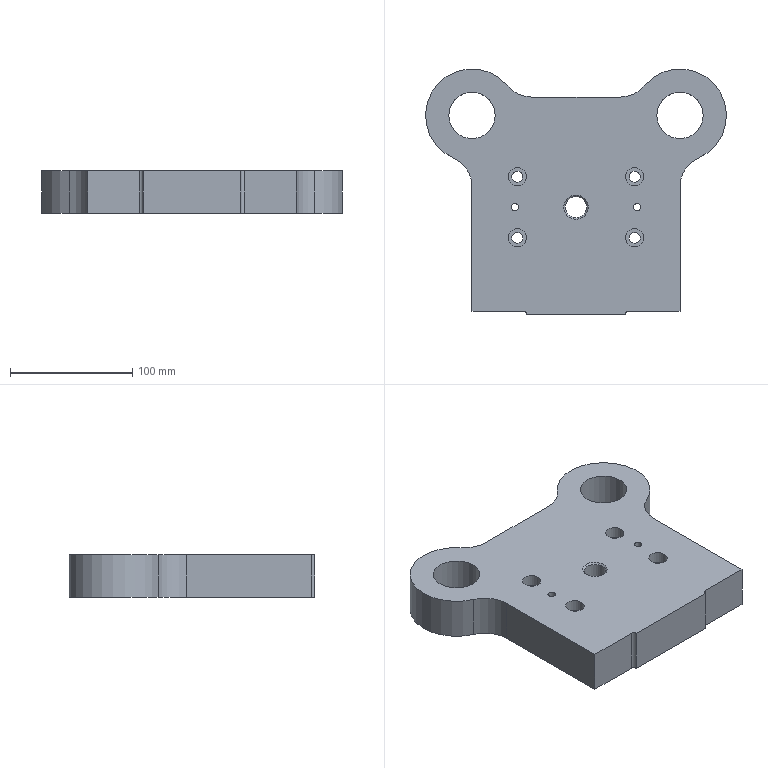Part | NX | features EXTRUDE 2, Radial Dimension 2, DATUM_CSYS 1, HOLE PACKAGE 1, SIMPLE HOLE 1, SYMBOLIC_THREAD 1 | 1 solid | 35 faces | box 246 x 201 x 35 mm | volume 1152139 mm3 | cylinder 21 | plane 12 | cone 2 | commonest cylinder face diameters 6 x4 9 x4 15 x4 50 x4 38 x2 76 x2
STEP:
#1=CARTESIAN_POINT('',(-43.5,-25.,0.));
#2=VERTEX_POINT('',#1);
#3=CARTESIAN_POINT('',(-48.,-25.,0.));
#4=DIRECTION('',(0.,0.,1.));
#5=DIRECTION('',(1.,0.,0.));
#6=AXIS2_PLACEMENT_3D('',#3,#4,#5);
#7=CIRCLE('',#6,4.5);
#8=EDGE_CURVE('',#2,#2,#7,.T.);
#9=ORIENTED_EDGE('',*,*,#8,.F.);
#10=EDGE_LOOP('',(#9));
#11=FACE_BOUND('',#10,.T.);
#12=CARTESIAN_POINT('',(-43.5,-25.,25.));
#13=VERTEX_POINT('',#12);
#14=CARTESIAN_POINT('',(-48.,-25.,25.));
#15=DIRECTION('',(0.,0.,1.));
#16=DIRECTION('',(1.,0.,0.));
#17=AXIS2_PLACEMENT_3D('',#14,#15,#16);
#18=CIRCLE('',#17,4.5);
#19=EDGE_CURVE('',#13,#13,#18,.T.);
#20=ORIENTED_EDGE('',*,*,#19,.T.);
#21=EDGE_LOOP('',(#20));
#22=FACE_BOUND('',#21,.T.);
#23=CARTESIAN_POINT('',(-48.,-25.,35.));
#24=DIRECTION('',(0.,0.,-1.));
#25=DIRECTION('',(-1.,0.,0.));
#26=AXIS2_PLACEMENT_3D('',#23,#24,#25);
#27=CYLINDRICAL_SURFACE('',#26,4.5);
#28=ADVANCED_FACE('',(#11,#22),#27,.F.);
#29=CARTESIAN_POINT('',(-43.5,25.,0.));
#30=VERTEX_POINT('',#29);
#31=CARTESIAN_POINT('',(-48.,25.,0.));
#32=DIRECTION('',(0.,0.,1.));
#33=DIRECTION('',(1.,0.,0.));
#34=AXIS2_PLACEMENT_3D('',#31,#32,#33);
#35=CIRCLE('',#34,4.5);
#36=EDGE_CURVE('',#30,#30,#35,.T.);
#37=ORIENTED_EDGE('',*,*,#36,.F.);
#38=EDGE_LOOP('',(#37));
#39=FACE_BOUND('',#38,.T.);
#40=CARTESIAN_POINT('',(-43.5,25.,25.));
#41=VERTEX_POINT('',#40);
#42=CARTESIAN_POINT('',(-48.,25.,25.));
#43=DIRECTION('',(0.,0.,1.));
#44=DIRECTION('',(1.,0.,0.));
#45=AXIS2_PLACEMENT_3D('',#42,#43,#44);
#46=CIRCLE('',#45,4.5);
#47=EDGE_CURVE('',#41,#41,#46,.T.);
#48=ORIENTED_EDGE('',*,*,#47,.T.);
#49=EDGE_LOOP('',(#48));
#50=FACE_BOUND('',#49,.T.);
#51=CARTESIAN_POINT('',(-48.,25.,35.));
#52=DIRECTION('',(0.,0.,-1.));
#53=DIRECTION('',(-1.,0.,0.));
#54=AXIS2_PLACEMENT_3D('',#51,#52,#53);
#55=CYLINDRICAL_SURFACE('',#54,4.5);
#56=ADVANCED_FACE('',(#39,#50),#55,.F.);
#57=CARTESIAN_POINT('',(52.5,-25.,0.));
#58=VERTEX_POINT('',#57);
#59=CARTESIAN_POINT('',(48.,-25.,0.));
#60=DIRECTION('',(0.,0.,1.));
#61=DIRECTION('',(1.,0.,0.));
#62=AXIS2_PLACEMENT_3D('',#59,#60,#61);
#63=CIRCLE('',#62,4.5);
#64=EDGE_CURVE('',#58,#58,#63,.T.);
#65=ORIENTED_EDGE('',*,*,#64,.F.);
#66=EDGE_LOOP('',(#65));
#67=FACE_BOUND('',#66,.T.);
#68=CARTESIAN_POINT('',(52.5,-25.,25.));
#69=VERTEX_POINT('',#68);
#70=CARTESIAN_POINT('',(48.,-25.,25.));
#71=DIRECTION('',(0.,0.,1.));
#72=DIRECTION('',(1.,0.,0.));
#73=AXIS2_PLACEMENT_3D('',#70,#71,#72);
#74=CIRCLE('',#73,4.5);
#75=EDGE_CURVE('',#69,#69,#74,.T.);
#76=ORIENTED_EDGE('',*,*,#75,.T.);
#77=EDGE_LOOP('',(#76));
#78=FACE_BOUND('',#77,.T.);
#79=CARTESIAN_POINT('',(48.,-25.,35.));
#80=DIRECTION('',(0.,0.,-1.));
#81=DIRECTION('',(-1.,0.,0.));
#82=AXIS2_PLACEMENT_3D('',#79,#80,#81);
#83=CYLINDRICAL_SURFACE('',#82,4.5);
#84=ADVANCED_FACE('',(#67,#78),#83,.F.);
#85=CARTESIAN_POINT('',(52.5,25.,0.));
#86=VERTEX_POINT('',#85);
#87=CARTESIAN_POINT('',(48.,25.,0.));
#88=DIRECTION('',(0.,0.,1.));
#89=DIRECTION('',(1.,0.,0.));
#90=AXIS2_PLACEMENT_3D('',#87,#88,#89);
#91=CIRCLE('',#90,4.5);
#92=EDGE_CURVE('',#86,#86,#91,.T.);
#93=ORIENTED_EDGE('',*,*,#92,.F.);
#94=EDGE_LOOP('',(#93));
#95=FACE_BOUND('',#94,.T.);
#96=CARTESIAN_POINT('',(52.5,25.,25.));
#97=VERTEX_POINT('',#96);
#98=CARTESIAN_POINT('',(48.,25.,25.));
#99=DIRECTION('',(0.,0.,1.));
#100=DIRECTION('',(1.,0.,0.));
#101=AXIS2_PLACEMENT_3D('',#98,#99,#100);
#102=CIRCLE('',#101,4.5);
#103=EDGE_CURVE('',#97,#97,#102,.T.);
#104=ORIENTED_EDGE('',*,*,#103,.T.);
#105=EDGE_LOOP('',(#104));
#106=FACE_BOUND('',#105,.T.);
#107=CARTESIAN_POINT('',(48.,25.,35.));
#108=DIRECTION('',(0.,0.,-1.));
#109=DIRECTION('',(-1.,0.,0.));
#110=AXIS2_PLACEMENT_3D('',#107,#108,#109);
#111=CYLINDRICAL_SURFACE('',#110,4.5);
#112=ADVANCED_FACE('',(#95,#106),#111,.F.);
#113=CARTESIAN_POINT('',(-85.,17.173,0.));
#114=VERTEX_POINT('',#113);
#115=CARTESIAN_POINT('',(-100.079,40.12,0.));
#116=VERTEX_POINT('',#115);
#117=CARTESIAN_POINT('',(-110.,17.173,0.));
#118=DIRECTION('',(0.,0.,1.));
#119=DIRECTION('',(1.,0.,0.));
#120=AXIS2_PLACEMENT_3D('',#117,#118,#119);
#121=CIRCLE('',#120,25.);
#122=EDGE_CURVE('',#114,#116,#121,.T.);
#123=ORIENTED_EDGE('',*,*,#122,.F.);
#124=CARTESIAN_POINT('',(-85.,17.173,35.));
#125=VERTEX_POINT('',#124);
#126=CARTESIAN_POINT('',(-85.,17.173,35.));
#127=DIRECTION('',(0.,0.,-1.));
#128=VECTOR('',#127,1000.);
#129=LINE('',#126,#128);
#130=EDGE_CURVE('',#125,#114,#129,.T.);
#131=ORIENTED_EDGE('',*,*,#130,.F.);
#132=CARTESIAN_POINT('',(-100.079,40.12,35.));
#133=VERTEX_POINT('',#132);
#134=CARTESIAN_POINT('',(-110.,17.173,35.));
#135=DIRECTION('',(0.,0.,1.));
#136=DIRECTION('',(1.,0.,0.));
#137=AXIS2_PLACEMENT_3D('',#134,#135,#136);
#138=CIRCLE('',#137,25.);
#139=EDGE_CURVE('',#125,#133,#138,.T.);
#140=ORIENTED_EDGE('',*,*,#139,.T.);
#141=CARTESIAN_POINT('',(-100.079,40.12,35.));
#142=DIRECTION('',(0.,0.,-1.));
#143=VECTOR('',#142,1000.);
#144=LINE('',#141,#143);
#145=EDGE_CURVE('',#133,#116,#144,.T.);
#146=ORIENTED_EDGE('',*,*,#145,.T.);
#147=EDGE_LOOP('',(#123,#131,#140,#146));
#148=FACE_BOUND('',#147,.T.);
#149=CARTESIAN_POINT('',(-110.,17.173,35.));
#150=DIRECTION('',(0.,0.,-1.));
#151=DIRECTION('',(-1.,0.,0.));
#152=AXIS2_PLACEMENT_3D('',#149,#150,#151);
#153=CYLINDRICAL_SURFACE('',#152,25.);
#154=ADVANCED_FACE('',(#148),#153,.F.);
#155=CARTESIAN_POINT('',(-55.642,99.127,0.));
#156=VERTEX_POINT('',#155);
#157=CARTESIAN_POINT('',(-85.,75.,0.));
#158=DIRECTION('',(0.,0.,-1.));
#159=DIRECTION('',(1.,0.,0.));
#160=AXIS2_PLACEMENT_3D('',#157,#158,#159);
#161=CIRCLE('',#160,38.);
#162=EDGE_CURVE('',#116,#156,#161,.T.);
#163=ORIENTED_EDGE('',*,*,#162,.F.);
#164=ORIENTED_EDGE('',*,*,#145,.F.);
#165=CARTESIAN_POINT('',(-55.642,99.127,35.));
#166=VERTEX_POINT('',#165);
#167=CARTESIAN_POINT('',(-85.,75.,35.));
#168=DIRECTION('',(0.,0.,-1.));
#169=DIRECTION('',(1.,0.,0.));
#170=AXIS2_PLACEMENT_3D('',#167,#168,#169);
#171=CIRCLE('',#170,38.);
#172=EDGE_CURVE('',#133,#166,#171,.T.);
#173=ORIENTED_EDGE('',*,*,#172,.T.);
#174=CARTESIAN_POINT('',(-55.642,99.127,35.));
#175=DIRECTION('',(0.,0.,-1.));
#176=VECTOR('',#175,1000.);
#177=LINE('',#174,#176);
#178=EDGE_CURVE('',#166,#156,#177,.T.);
#179=ORIENTED_EDGE('',*,*,#178,.T.);
#180=EDGE_LOOP('',(#163,#164,#173,#179));
#181=FACE_BOUND('',#180,.T.);
#182=CARTESIAN_POINT('',(-85.,75.,35.));
#183=DIRECTION('',(0.,0.,-1.));
#184=DIRECTION('',(-1.,0.,0.));
#185=AXIS2_PLACEMENT_3D('',#182,#183,#184);
#186=CYLINDRICAL_SURFACE('',#185,38.);
#187=ADVANCED_FACE('',(#181),#186,.T.);
#188=CARTESIAN_POINT('',(-36.328,90.,0.));
#189=VERTEX_POINT('',#188);
#190=CARTESIAN_POINT('',(-36.328,115.,0.));
#191=DIRECTION('',(0.,0.,1.));
#192=DIRECTION('',(1.,0.,0.));
#193=AXIS2_PLACEMENT_3D('',#190,#191,#192);
#194=CIRCLE('',#193,25.);
#195=EDGE_CURVE('',#156,#189,#194,.T.);
#196=ORIENTED_EDGE('',*,*,#195,.F.);
#197=ORIENTED_EDGE('',*,*,#178,.F.);
#198=CARTESIAN_POINT('',(-36.328,90.,35.));
#199=VERTEX_POINT('',#198);
#200=CARTESIAN_POINT('',(-36.328,115.,35.));
#201=DIRECTION('',(0.,0.,1.));
#202=DIRECTION('',(1.,0.,0.));
#203=AXIS2_PLACEMENT_3D('',#200,#201,#202);
#204=CIRCLE('',#203,25.);
#205=EDGE_CURVE('',#166,#199,#204,.T.);
#206=ORIENTED_EDGE('',*,*,#205,.T.);
#207=CARTESIAN_POINT('',(-36.328,90.,35.));
#208=DIRECTION('',(0.,0.,-1.));
#209=VECTOR('',#208,1000.);
#210=LINE('',#207,#209);
#211=EDGE_CURVE('',#199,#189,#210,.T.);
#212=ORIENTED_EDGE('',*,*,#211,.T.);
#213=EDGE_LOOP('',(#196,#197,#206,#212));
#214=FACE_BOUND('',#213,.T.);
#215=CARTESIAN_POINT('',(-36.328,115.,35.));
#216=DIRECTION('',(0.,0.,-1.));
#217=DIRECTION('',(-1.,0.,0.));
#218=AXIS2_PLACEMENT_3D('',#215,#216,#217);
#219=CYLINDRICAL_SURFACE('',#218,25.);
#220=ADVANCED_FACE('',(#214),#219,.F.);
#221=CARTESIAN_POINT('',(36.328,90.,0.));
#222=VERTEX_POINT('',#221);
#223=CARTESIAN_POINT('',(-36.328,90.,0.));
#224=DIRECTION('',(1.,0.,0.));
#225=VECTOR('',#224,1000.);
#226=LINE('',#223,#225);
#227=EDGE_CURVE('',#189,#222,#226,.T.);
#228=ORIENTED_EDGE('',*,*,#227,.F.);
#229=ORIENTED_EDGE('',*,*,#211,.F.);
#230=CARTESIAN_POINT('',(36.328,90.,35.));
#231=VERTEX_POINT('',#230);
#232=CARTESIAN_POINT('',(-36.328,90.,35.));
#233=DIRECTION('',(1.,0.,0.));
#234=VECTOR('',#233,1000.);
#235=LINE('',#232,#234);
#236=EDGE_CURVE('',#199,#231,#235,.T.);
#237=ORIENTED_EDGE('',*,*,#236,.T.);
#238=CARTESIAN_POINT('',(36.328,90.,35.));
#239=DIRECTION('',(0.,0.,-1.));
#240=VECTOR('',#239,1000.);
#241=LINE('',#238,#240);
#242=EDGE_CURVE('',#231,#222,#241,.T.);
#243=ORIENTED_EDGE('',*,*,#242,.T.);
#244=EDGE_LOOP('',(#228,#229,#237,#243));
#245=FACE_BOUND('',#244,.T.);
#246=CARTESIAN_POINT('',(-36.328,90.,35.));
#247=DIRECTION('',(0.,1.,0.));
#248=DIRECTION('',(0.,0.,1.));
#249=AXIS2_PLACEMENT_3D('',#246,#247,#248);
#250=PLANE('',#249);
#251=ADVANCED_FACE('',(#245),#250,.T.);
#252=CARTESIAN_POINT('',(55.642,99.127,0.));
#253=VERTEX_POINT('',#252);
#254=CARTESIAN_POINT('',(36.328,115.,0.));
#255=DIRECTION('',(0.,0.,1.));
#256=DIRECTION('',(1.,0.,0.));
#257=AXIS2_PLACEMENT_3D('',#254,#255,#256);
#258=CIRCLE('',#257,25.);
#259=EDGE_CURVE('',#222,#253,#258,.T.);
#260=ORIENTED_EDGE('',*,*,#259,.F.);
#261=ORIENTED_EDGE('',*,*,#242,.F.);
#262=CARTESIAN_POINT('',(55.642,99.127,35.));
#263=VERTEX_POINT('',#262);
#264=CARTESIAN_POINT('',(36.328,115.,35.));
#265=DIRECTION('',(0.,0.,1.));
#266=DIRECTION('',(1.,0.,0.));
#267=AXIS2_PLACEMENT_3D('',#264,#265,#266);
#268=CIRCLE('',#267,25.);
#269=EDGE_CURVE('',#231,#263,#268,.T.);
#270=ORIENTED_EDGE('',*,*,#269,.T.);
#271=CARTESIAN_POINT('',(55.642,99.127,35.));
#272=DIRECTION('',(0.,0.,-1.));
#273=VECTOR('',#272,1000.);
#274=LINE('',#271,#273);
#275=EDGE_CURVE('',#263,#253,#274,.T.);
#276=ORIENTED_EDGE('',*,*,#275,.T.);
#277=EDGE_LOOP('',(#260,#261,#270,#276));
#278=FACE_BOUND('',#277,.T.);
#279=CARTESIAN_POINT('',(36.328,115.,35.));
#280=DIRECTION('',(0.,0.,-1.));
#281=DIRECTION('',(-1.,0.,0.));
#282=AXIS2_PLACEMENT_3D('',#279,#280,#281);
#283=CYLINDRICAL_SURFACE('',#282,25.);
#284=ADVANCED_FACE('',(#278),#283,.F.);
#285=CARTESIAN_POINT('',(100.079,40.12,0.));
#286=VERTEX_POINT('',#285);
#287=CARTESIAN_POINT('',(85.,75.,0.));
#288=DIRECTION('',(0.,0.,-1.));
#289=DIRECTION('',(1.,0.,0.));
#290=AXIS2_PLACEMENT_3D('',#287,#288,#289);
#291=CIRCLE('',#290,38.);
#292=EDGE_CURVE('',#253,#286,#291,.T.);
#293=ORIENTED_EDGE('',*,*,#292,.F.);
#294=ORIENTED_EDGE('',*,*,#275,.F.);
#295=CARTESIAN_POINT('',(100.079,40.12,35.));
#296=VERTEX_POINT('',#295);
#297=CARTESIAN_POINT('',(85.,75.,35.));
#298=DIRECTION('',(0.,0.,-1.));
#299=DIRECTION('',(1.,0.,0.));
#300=AXIS2_PLACEMENT_3D('',#297,#298,#299);
#301=CIRCLE('',#300,38.);
#302=EDGE_CURVE('',#263,#296,#301,.T.);
#303=ORIENTED_EDGE('',*,*,#302,.T.);
#304=CARTESIAN_POINT('',(100.079,40.12,35.));
#305=DIRECTION('',(0.,0.,-1.));
#306=VECTOR('',#305,1000.);
#307=LINE('',#304,#306);
#308=EDGE_CURVE('',#296,#286,#307,.T.);
#309=ORIENTED_EDGE('',*,*,#308,.T.);
#310=EDGE_LOOP('',(#293,#294,#303,#309));
#311=FACE_BOUND('',#310,.T.);
#312=CARTESIAN_POINT('',(85.,75.,35.));
#313=DIRECTION('',(0.,0.,-1.));
#314=DIRECTION('',(-1.,0.,0.));
#315=AXIS2_PLACEMENT_3D('',#312,#313,#314);
#316=CYLINDRICAL_SURFACE('',#315,38.);
#317=ADVANCED_FACE('',(#311),#316,.T.);
#318=CARTESIAN_POINT('',(85.,17.173,0.));
#319=VERTEX_POINT('',#318);
#320=CARTESIAN_POINT('',(110.,17.173,0.));
#321=DIRECTION('',(0.,0.,1.));
#322=DIRECTION('',(1.,0.,0.));
#323=AXIS2_PLACEMENT_3D('',#320,#321,#322);
#324=CIRCLE('',#323,25.);
#325=EDGE_CURVE('',#286,#319,#324,.T.);
#326=ORIENTED_EDGE('',*,*,#325,.F.);
#327=ORIENTED_EDGE('',*,*,#308,.F.);
#328=CARTESIAN_POINT('',(85.,17.173,35.));
#329=VERTEX_POINT('',#328);
#330=CARTESIAN_POINT('',(110.,17.173,35.));
#331=DIRECTION('',(0.,0.,1.));
#332=DIRECTION('',(1.,0.,0.));
#333=AXIS2_PLACEMENT_3D('',#330,#331,#332);
#334=CIRCLE('',#333,25.);
#335=EDGE_CURVE('',#296,#329,#334,.T.);
#336=ORIENTED_EDGE('',*,*,#335,.T.);
#337=CARTESIAN_POINT('',(85.,17.173,35.));
#338=DIRECTION('',(0.,0.,-1.));
#339=VECTOR('',#338,1000.);
#340=LINE('',#337,#339);
#341=EDGE_CURVE('',#329,#319,#340,.T.);
#342=ORIENTED_EDGE('',*,*,#341,.T.);
#343=EDGE_LOOP('',(#326,#327,#336,#342));
#344=FACE_BOUND('',#343,.T.);
#345=CARTESIAN_POINT('',(110.,17.173,35.));
#346=DIRECTION('',(0.,0.,-1.));
#347=DIRECTION('',(-1.,0.,0.));
#348=AXIS2_PLACEMENT_3D('',#345,#346,#347);
#349=CYLINDRICAL_SURFACE('',#348,25.);
#350=ADVANCED_FACE('',(#344),#349,.F.);
#351=CARTESIAN_POINT('',(85.,-85.,0.));
#352=VERTEX_POINT('',#351);
#353=CARTESIAN_POINT('',(85.,17.173,0.));
#354=DIRECTION('',(0.,-1.,0.));
#355=VECTOR('',#354,1000.);
#356=LINE('',#353,#355);
#357=EDGE_CURVE('',#319,#352,#356,.T.);
#358=ORIENTED_EDGE('',*,*,#357,.F.);
#359=ORIENTED_EDGE('',*,*,#341,.F.);
#360=CARTESIAN_POINT('',(85.,-85.,35.));
#361=VERTEX_POINT('',#360);
#362=CARTESIAN_POINT('',(85.,17.173,35.));
#363=DIRECTION('',(0.,-1.,0.));
#364=VECTOR('',#363,1000.);
#365=LINE('',#362,#364);
#366=EDGE_CURVE('',#329,#361,#365,.T.);
#367=ORIENTED_EDGE('',*,*,#366,.T.);
#368=CARTESIAN_POINT('',(85.,-85.,35.));
#369=DIRECTION('',(0.,0.,-1.));
#370=VECTOR('',#369,1000.);
#371=LINE('',#368,#370);
#372=EDGE_CURVE('',#361,#352,#371,.T.);
#373=ORIENTED_EDGE('',*,*,#372,.T.);
#374=EDGE_LOOP('',(#358,#359,#367,#373));
#375=FACE_BOUND('',#374,.T.);
#376=CARTESIAN_POINT('',(85.,17.173,35.));
#377=DIRECTION('',(1.,0.,0.));
#378=DIRECTION('',(0.,0.,-1.));
#379=AXIS2_PLACEMENT_3D('',#376,#377,#378);
#380=PLANE('',#379);
#381=ADVANCED_FACE('',(#375),#380,.T.);
#382=CARTESIAN_POINT('',(43.,-85.,0.));
#383=VERTEX_POINT('',#382);
#384=CARTESIAN_POINT('',(85.,-85.,0.));
#385=DIRECTION('',(-1.,0.,0.));
#386=VECTOR('',#385,1000.);
#387=LINE('',#384,#386);
#388=EDGE_CURVE('',#352,#383,#387,.T.);
#389=ORIENTED_EDGE('',*,*,#388,.F.);
#390=ORIENTED_EDGE('',*,*,#372,.F.);
#391=CARTESIAN_POINT('',(43.,-85.,35.));
#392=VERTEX_POINT('',#391);
#393=CARTESIAN_POINT('',(85.,-85.,35.));
#394=DIRECTION('',(-1.,0.,0.));
#395=VECTOR('',#394,1000.);
#396=LINE('',#393,#395);
#397=EDGE_CURVE('',#361,#392,#396,.T.);
#398=ORIENTED_EDGE('',*,*,#397,.T.);
#399=CARTESIAN_POINT('',(43.,-85.,35.));
#400=DIRECTION('',(0.,0.,-1.));
#401=VECTOR('',#400,1000.);
#402=LINE('',#399,#401);
#403=EDGE_CURVE('',#392,#383,#402,.T.);
#404=ORIENTED_EDGE('',*,*,#403,.T.);
#405=EDGE_LOOP('',(#389,#390,#398,#404));
#406=FACE_BOUND('',#405,.T.);
#407=CARTESIAN_POINT('',(85.,-85.,35.));
#408=DIRECTION('',(0.,-1.,0.));
#409=DIRECTION('',(0.,0.,-1.));
#410=AXIS2_PLACEMENT_3D('',#407,#408,#409);
#411=PLANE('',#410);
#412=ADVANCED_FACE('',(#406),#411,.T.);
#413=CARTESIAN_POINT('',(40.,-88.,0.));
#414=VERTEX_POINT('',#413);
#415=CARTESIAN_POINT('',(43.,-88.,0.));
#416=DIRECTION('',(0.,0.,1.));
#417=DIRECTION('',(1.,0.,0.));
#418=AXIS2_PLACEMENT_3D('',#415,#416,#417);
#419=CIRCLE('',#418,3.);
#420=EDGE_CURVE('',#383,#414,#419,.T.);
#421=ORIENTED_EDGE('',*,*,#420,.F.);
#422=ORIENTED_EDGE('',*,*,#403,.F.);
#423=CARTESIAN_POINT('',(40.,-88.,35.));
#424=VERTEX_POINT('',#423);
#425=CARTESIAN_POINT('',(43.,-88.,35.));
#426=DIRECTION('',(0.,0.,1.));
#427=DIRECTION('',(1.,0.,0.));
#428=AXIS2_PLACEMENT_3D('',#425,#426,#427);
#429=CIRCLE('',#428,3.);
#430=EDGE_CURVE('',#392,#424,#429,.T.);
#431=ORIENTED_EDGE('',*,*,#430,.T.);
#432=CARTESIAN_POINT('',(40.,-88.,35.));
#433=DIRECTION('',(0.,0.,-1.));
#434=VECTOR('',#433,1000.);
#435=LINE('',#432,#434);
#436=EDGE_CURVE('',#424,#414,#435,.T.);
#437=ORIENTED_EDGE('',*,*,#436,.T.);
#438=EDGE_LOOP('',(#421,#422,#431,#437));
#439=FACE_BOUND('',#438,.T.);
#440=CARTESIAN_POINT('',(43.,-88.,35.));
#441=DIRECTION('',(0.,0.,-1.));
#442=DIRECTION('',(-1.,0.,0.));
#443=AXIS2_PLACEMENT_3D('',#440,#441,#442);
#444=CYLINDRICAL_SURFACE('',#443,3.);
#445=ADVANCED_FACE('',(#439),#444,.F.);
#446=CARTESIAN_POINT('',(-40.,-88.,0.));
#447=VERTEX_POINT('',#446);
#448=CARTESIAN_POINT('',(40.,-88.,0.));
#449=DIRECTION('',(-1.,0.,0.));
#450=VECTOR('',#449,1000.);
#451=LINE('',#448,#450);
#452=EDGE_CURVE('',#414,#447,#451,.T.);
#453=ORIENTED_EDGE('',*,*,#452,.F.);
#454=ORIENTED_EDGE('',*,*,#436,.F.);
#455=CARTESIAN_POINT('',(-40.,-88.,35.));
#456=VERTEX_POINT('',#455);
#457=CARTESIAN_POINT('',(40.,-88.,35.));
#458=DIRECTION('',(-1.,0.,0.));
#459=VECTOR('',#458,1000.);
#460=LINE('',#457,#459);
#461=EDGE_CURVE('',#424,#456,#460,.T.);
#462=ORIENTED_EDGE('',*,*,#461,.T.);
#463=CARTESIAN_POINT('',(-40.,-88.,35.));
#464=DIRECTION('',(0.,0.,-1.));
#465=VECTOR('',#464,1000.);
#466=LINE('',#463,#465);
#467=EDGE_CURVE('',#456,#447,#466,.T.);
#468=ORIENTED_EDGE('',*,*,#467,.T.);
#469=EDGE_LOOP('',(#453,#454,#462,#468));
#470=FACE_BOUND('',#469,.T.);
#471=CARTESIAN_POINT('',(40.,-88.,35.));
#472=DIRECTION('',(0.,-1.,0.));
#473=DIRECTION('',(0.,0.,-1.));
#474=AXIS2_PLACEMENT_3D('',#471,#472,#473);
#475=PLANE('',#474);
#476=ADVANCED_FACE('',(#470),#475,.T.);
#477=CARTESIAN_POINT('',(-43.,-85.,0.));
#478=VERTEX_POINT('',#477);
#479=CARTESIAN_POINT('',(-43.,-88.,0.));
#480=DIRECTION('',(0.,0.,1.));
#481=DIRECTION('',(1.,0.,0.));
#482=AXIS2_PLACEMENT_3D('',#479,#480,#481);
#483=CIRCLE('',#482,3.);
#484=EDGE_CURVE('',#447,#478,#483,.T.);
#485=ORIENTED_EDGE('',*,*,#484,.F.);
#486=ORIENTED_EDGE('',*,*,#467,.F.);
#487=CARTESIAN_POINT('',(-43.,-85.,35.));
#488=VERTEX_POINT('',#487);
#489=CARTESIAN_POINT('',(-43.,-88.,35.));
#490=DIRECTION('',(0.,0.,1.));
#491=DIRECTION('',(1.,0.,0.));
#492=AXIS2_PLACEMENT_3D('',#489,#490,#491);
#493=CIRCLE('',#492,3.);
#494=EDGE_CURVE('',#456,#488,#493,.T.);
#495=ORIENTED_EDGE('',*,*,#494,.T.);
#496=CARTESIAN_POINT('',(-43.,-85.,35.));
#497=DIRECTION('',(0.,0.,-1.));
#498=VECTOR('',#497,1000.);
#499=LINE('',#496,#498);
#500=EDGE_CURVE('',#488,#478,#499,.T.);
#501=ORIENTED_EDGE('',*,*,#500,.T.);
#502=EDGE_LOOP('',(#485,#486,#495,#501));
#503=FACE_BOUND('',#502,.T.);
#504=CARTESIAN_POINT('',(-43.,-88.,35.));
#505=DIRECTION('',(0.,0.,-1.));
#506=DIRECTION('',(-1.,0.,0.));
#507=AXIS2_PLACEMENT_3D('',#504,#505,#506);
#508=CYLINDRICAL_SURFACE('',#507,3.);
#509=ADVANCED_FACE('',(#503),#508,.F.);
#510=CARTESIAN_POINT('',(-85.,-85.,0.));
#511=VERTEX_POINT('',#510);
#512=CARTESIAN_POINT('',(-43.,-85.,0.));
#513=DIRECTION('',(-1.,0.,0.));
#514=VECTOR('',#513,1000.);
#515=LINE('',#512,#514);
#516=EDGE_CURVE('',#478,#511,#515,.T.);
#517=ORIENTED_EDGE('',*,*,#516,.F.);
#518=ORIENTED_EDGE('',*,*,#500,.F.);
#519=CARTESIAN_POINT('',(-85.,-85.,35.));
#520=VERTEX_POINT('',#519);
#521=CARTESIAN_POINT('',(-43.,-85.,35.));
#522=DIRECTION('',(-1.,0.,0.));
#523=VECTOR('',#522,1000.);
#524=LINE('',#521,#523);
#525=EDGE_CURVE('',#488,#520,#524,.T.);
#526=ORIENTED_EDGE('',*,*,#525,.T.);
#527=CARTESIAN_POINT('',(-85.,-85.,35.));
#528=DIRECTION('',(0.,0.,-1.));
#529=VECTOR('',#528,1000.);
#530=LINE('',#527,#529);
#531=EDGE_CURVE('',#520,#511,#530,.T.);
#532=ORIENTED_EDGE('',*,*,#531,.T.);
#533=EDGE_LOOP('',(#517,#518,#526,#532));
#534=FACE_BOUND('',#533,.T.);
#535=CARTESIAN_POINT('',(-43.,-85.,35.));
#536=DIRECTION('',(0.,-1.,0.));
#537=DIRECTION('',(0.,0.,-1.));
#538=AXIS2_PLACEMENT_3D('',#535,#536,#537);
#539=PLANE('',#538);
#540=ADVANCED_FACE('',(#534),#539,.T.);
#541=CARTESIAN_POINT('',(-47.,0.,35.));
#542=VERTEX_POINT('',#541);
#543=CARTESIAN_POINT('',(-50.,0.,35.));
#544=DIRECTION('',(0.,0.,1.));
#545=DIRECTION('',(1.,0.,0.));
#546=AXIS2_PLACEMENT_3D('',#543,#544,#545);
#547=CIRCLE('',#546,3.);
#548=EDGE_CURVE('',#542,#542,#547,.T.);
#549=ORIENTED_EDGE('',*,*,#548,.T.);
#550=EDGE_LOOP('',(#549));
#551=FACE_BOUND('',#550,.T.);
#552=CARTESIAN_POINT('',(-47.,0.,0.));
#553=VERTEX_POINT('',#552);
#554=CARTESIAN_POINT('',(-50.,0.,0.));
#555=DIRECTION('',(0.,0.,1.));
#556=DIRECTION('',(1.,0.,0.));
#557=AXIS2_PLACEMENT_3D('',#554,#555,#556);
#558=CIRCLE('',#557,3.);
#559=EDGE_CURVE('',#553,#553,#558,.T.);
#560=ORIENTED_EDGE('',*,*,#559,.F.);
#561=EDGE_LOOP('',(#560));
#562=FACE_BOUND('',#561,.T.);
#563=CARTESIAN_POINT('',(-50.,0.,35.));
#564=DIRECTION('',(0.,0.,-1.));
#565=DIRECTION('',(-1.,0.,0.));
#566=AXIS2_PLACEMENT_3D('',#563,#564,#565);
#567=CYLINDRICAL_SURFACE('',#566,3.);
#568=ADVANCED_FACE('',(#551,#562),#567,.F.);
#569=CARTESIAN_POINT('',(53.,0.,35.));
#570=VERTEX_POINT('',#569);
#571=CARTESIAN_POINT('',(50.,0.,35.));
#572=DIRECTION('',(0.,0.,1.));
#573=DIRECTION('',(1.,0.,0.));
#574=AXIS2_PLACEMENT_3D('',#571,#572,#573);
#575=CIRCLE('',#574,3.);
#576=EDGE_CURVE('',#570,#570,#575,.T.);
#577=ORIENTED_EDGE('',*,*,#576,.T.);
#578=EDGE_LOOP('',(#577));
#579=FACE_BOUND('',#578,.T.);
#580=CARTESIAN_POINT('',(53.,0.,0.));
#581=VERTEX_POINT('',#580);
#582=CARTESIAN_POINT('',(50.,0.,0.));
#583=DIRECTION('',(0.,0.,1.));
#584=DIRECTION('',(1.,0.,0.));
#585=AXIS2_PLACEMENT_3D('',#582,#583,#584);
#586=CIRCLE('',#585,3.);
#587=EDGE_CURVE('',#581,#581,#586,.T.);
#588=ORIENTED_EDGE('',*,*,#587,.F.);
#589=EDGE_LOOP('',(#588));
#590=FACE_BOUND('',#589,.T.);
#591=CARTESIAN_POINT('',(50.,0.,35.));
#592=DIRECTION('',(0.,0.,-1.));
#593=DIRECTION('',(-1.,0.,0.));
#594=AXIS2_PLACEMENT_3D('',#591,#592,#593);
#595=CYLINDRICAL_SURFACE('',#594,3.);
#596=ADVANCED_FACE('',(#579,#590),#595,.F.);
#597=CARTESIAN_POINT('',(104.,75.,35.));
#598=VERTEX_POINT('',#597);
#599=CARTESIAN_POINT('',(85.,75.,35.));
#600=DIRECTION('',(0.,0.,1.));
#601=DIRECTION('',(1.,0.,0.));
#602=AXIS2_PLACEMENT_3D('',#599,#600,#601);
#603=CIRCLE('',#602,19.);
#604=EDGE_CURVE('',#598,#598,#603,.T.);
#605=ORIENTED_EDGE('',*,*,#604,.T.);
#606=EDGE_LOOP('',(#605));
#607=FACE_BOUND('',#606,.T.);
#608=CARTESIAN_POINT('',(104.,75.,0.));
#609=VERTEX_POINT('',#608);
#610=CARTESIAN_POINT('',(85.,75.,0.));
#611=DIRECTION('',(0.,0.,1.));
#612=DIRECTION('',(1.,0.,0.));
#613=AXIS2_PLACEMENT_3D('',#610,#611,#612);
#614=CIRCLE('',#613,19.);
#615=EDGE_CURVE('',#609,#609,#614,.T.);
#616=ORIENTED_EDGE('',*,*,#615,.F.);
#617=EDGE_LOOP('',(#616));
#618=FACE_BOUND('',#617,.T.);
#619=CARTESIAN_POINT('',(85.,75.,35.));
#620=DIRECTION('',(0.,0.,-1.));
#621=DIRECTION('',(-1.,0.,0.));
#622=AXIS2_PLACEMENT_3D('',#619,#620,#621);
#623=CYLINDRICAL_SURFACE('',#622,19.);
#624=ADVANCED_FACE('',(#607,#618),#623,.F.);
#625=CARTESIAN_POINT('',(-85.,-85.,0.));
#626=DIRECTION('',(0.,1.,0.));
#627=VECTOR('',#626,1000.);
#628=LINE('',#625,#627);
#629=EDGE_CURVE('',#511,#114,#628,.T.);
#630=ORIENTED_EDGE('',*,*,#629,.F.);
#631=ORIENTED_EDGE('',*,*,#531,.F.);
#632=CARTESIAN_POINT('',(-85.,-85.,35.));
#633=DIRECTION('',(0.,1.,0.));
#634=VECTOR('',#633,1000.);
#635=LINE('',#632,#634);
#636=EDGE_CURVE('',#520,#125,#635,.T.);
#637=ORIENTED_EDGE('',*,*,#636,.T.);
#638=ORIENTED_EDGE('',*,*,#130,.T.);
#639=EDGE_LOOP('',(#630,#631,#637,#638));
#640=FACE_BOUND('',#639,.T.);
#641=CARTESIAN_POINT('',(-85.,-85.,35.));
#642=DIRECTION('',(-1.,0.,0.));
#643=DIRECTION('',(0.,0.,1.));
#644=AXIS2_PLACEMENT_3D('',#641,#642,#643);
#645=PLANE('',#644);
#646=ADVANCED_FACE('',(#640),#645,.T.);
#647=CARTESIAN_POINT('',(-66.,75.,35.));
#648=VERTEX_POINT('',#647);
#649=CARTESIAN_POINT('',(-85.,75.,35.));
#650=DIRECTION('',(0.,0.,1.));
#651=DIRECTION('',(1.,0.,0.));
#652=AXIS2_PLACEMENT_3D('',#649,#650,#651);
#653=CIRCLE('',#652,19.);
#654=EDGE_CURVE('',#648,#648,#653,.T.);
#655=ORIENTED_EDGE('',*,*,#654,.T.);
#656=EDGE_LOOP('',(#655));
#657=FACE_BOUND('',#656,.T.);
#658=CARTESIAN_POINT('',(-66.,75.,0.));
#659=VERTEX_POINT('',#658);
#660=CARTESIAN_POINT('',(-85.,75.,0.));
#661=DIRECTION('',(0.,0.,1.));
#662=DIRECTION('',(1.,0.,0.));
#663=AXIS2_PLACEMENT_3D('',#660,#661,#662);
#664=CIRCLE('',#663,19.);
#665=EDGE_CURVE('',#659,#659,#664,.T.);
#666=ORIENTED_EDGE('',*,*,#665,.F.);
#667=EDGE_LOOP('',(#666));
#668=FACE_BOUND('',#667,.T.);
#669=CARTESIAN_POINT('',(-85.,75.,35.));
#670=DIRECTION('',(0.,0.,-1.));
#671=DIRECTION('',(-1.,0.,0.));
#672=AXIS2_PLACEMENT_3D('',#669,#670,#671);
#673=CYLINDRICAL_SURFACE('',#672,19.);
#674=ADVANCED_FACE('',(#657,#668),#673,.F.);
#675=CARTESIAN_POINT('',(10.,0.,35.));
#676=VERTEX_POINT('',#675);
#677=CARTESIAN_POINT('',(0.,0.,35.));
#678=DIRECTION('',(0.,0.,1.));
#679=DIRECTION('',(1.,0.,0.));
#680=AXIS2_PLACEMENT_3D('',#677,#678,#679);
#681=CIRCLE('',#680,10.);
#682=EDGE_CURVE('',#676,#676,#681,.F.);
#683=ORIENTED_EDGE('',*,*,#682,.T.);
#684=EDGE_LOOP('',(#683));
#685=FACE_BOUND('',#684,.T.);
#686=CARTESIAN_POINT('',(55.5,-25.,35.));
#687=VERTEX_POINT('',#686);
#688=CARTESIAN_POINT('',(48.,-25.,35.));
#689=DIRECTION('',(0.,0.,1.));
#690=DIRECTION('',(1.,0.,0.));
#691=AXIS2_PLACEMENT_3D('',#688,#689,#690);
#692=CIRCLE('',#691,7.5);
#693=EDGE_CURVE('',#687,#687,#692,.T.);
#694=ORIENTED_EDGE('',*,*,#693,.F.);
#695=EDGE_LOOP('',(#694));
#696=FACE_BOUND('',#695,.T.);
#697=CARTESIAN_POINT('',(-40.5,25.,35.));
#698=VERTEX_POINT('',#697);
#699=CARTESIAN_POINT('',(-48.,25.,35.));
#700=DIRECTION('',(0.,0.,1.));
#701=DIRECTION('',(1.,0.,0.));
#702=AXIS2_PLACEMENT_3D('',#699,#700,#701);
#703=CIRCLE('',#702,7.5);
#704=EDGE_CURVE('',#698,#698,#703,.T.);
#705=ORIENTED_EDGE('',*,*,#704,.F.);
#706=EDGE_LOOP('',(#705));
#707=FACE_BOUND('',#706,.T.);
#708=CARTESIAN_POINT('',(-40.5,-25.,35.));
#709=VERTEX_POINT('',#708);
#710=CARTESIAN_POINT('',(-48.,-25.,35.));
#711=DIRECTION('',(0.,0.,1.));
#712=DIRECTION('',(1.,0.,0.));
#713=AXIS2_PLACEMENT_3D('',#710,#711,#712);
#714=CIRCLE('',#713,7.5);
#715=EDGE_CURVE('',#709,#709,#714,.T.);
#716=ORIENTED_EDGE('',*,*,#715,.F.);
#717=EDGE_LOOP('',(#716));
#718=FACE_BOUND('',#717,.T.);
#719=CARTESIAN_POINT('',(55.5,25.,35.));
#720=VERTEX_POINT('',#719);
#721=CARTESIAN_POINT('',(48.,25.,35.));
#722=DIRECTION('',(0.,0.,1.));
#723=DIRECTION('',(1.,0.,0.));
#724=AXIS2_PLACEMENT_3D('',#721,#722,#723);
#725=CIRCLE('',#724,7.5);
#726=EDGE_CURVE('',#720,#720,#725,.T.);
#727=ORIENTED_EDGE('',*,*,#726,.F.);
#728=EDGE_LOOP('',(#727));
#729=FACE_BOUND('',#728,.T.);
#730=ORIENTED_EDGE('',*,*,#139,.F.);
#731=ORIENTED_EDGE('',*,*,#636,.F.);
#732=ORIENTED_EDGE('',*,*,#525,.F.);
#733=ORIENTED_EDGE('',*,*,#494,.F.);
#734=ORIENTED_EDGE('',*,*,#461,.F.);
#735=ORIENTED_EDGE('',*,*,#430,.F.);
#736=ORIENTED_EDGE('',*,*,#397,.F.);
#737=ORIENTED_EDGE('',*,*,#366,.F.);
#738=ORIENTED_EDGE('',*,*,#335,.F.);
#739=ORIENTED_EDGE('',*,*,#302,.F.);
#740=ORIENTED_EDGE('',*,*,#269,.F.);
#741=ORIENTED_EDGE('',*,*,#236,.F.);
#742=ORIENTED_EDGE('',*,*,#205,.F.);
#743=ORIENTED_EDGE('',*,*,#172,.F.);
#744=EDGE_LOOP('',(#730,#731,#732,#733,#734,#735,#736,#737,#738,#739,#740,#741,#742,#743));
#745=FACE_BOUND('',#744,.T.);
#746=ORIENTED_EDGE('',*,*,#604,.F.);
#747=EDGE_LOOP('',(#746));
#748=FACE_BOUND('',#747,.T.);
#749=ORIENTED_EDGE('',*,*,#576,.F.);
#750=EDGE_LOOP('',(#749));
#751=FACE_BOUND('',#750,.T.);
#752=ORIENTED_EDGE('',*,*,#548,.F.);
#753=EDGE_LOOP('',(#752));
#754=FACE_BOUND('',#753,.T.);
#755=ORIENTED_EDGE('',*,*,#654,.F.);
#756=EDGE_LOOP('',(#755));
#757=FACE_BOUND('',#756,.T.);
#758=CARTESIAN_POINT('',(-110.,17.173,35.));
#759=DIRECTION('',(0.,0.,1.));
#760=DIRECTION('',(1.,0.,0.));
#761=AXIS2_PLACEMENT_3D('',#758,#759,#760);
#762=PLANE('',#761);
#763=ADVANCED_FACE('',(#685,#696,#707,#718,#729,#745,#748,#751,#754,#757),#762,.T.);
#764=CARTESIAN_POINT('',(10.,0.,0.));
#765=VERTEX_POINT('',#764);
#766=CARTESIAN_POINT('',(0.,0.,0.));
#767=DIRECTION('',(0.,0.,1.));
#768=DIRECTION('',(1.,0.,0.));
#769=AXIS2_PLACEMENT_3D('',#766,#767,#768);
#770=CIRCLE('',#769,10.);
#771=EDGE_CURVE('',#765,#765,#770,.T.);
#772=ORIENTED_EDGE('',*,*,#771,.T.);
#773=EDGE_LOOP('',(#772));
#774=FACE_BOUND('',#773,.T.);
#775=ORIENTED_EDGE('',*,*,#122,.T.);
#776=ORIENTED_EDGE('',*,*,#162,.T.);
#777=ORIENTED_EDGE('',*,*,#195,.T.);
#778=ORIENTED_EDGE('',*,*,#227,.T.);
#779=ORIENTED_EDGE('',*,*,#259,.T.);
#780=ORIENTED_EDGE('',*,*,#292,.T.);
#781=ORIENTED_EDGE('',*,*,#325,.T.);
#782=ORIENTED_EDGE('',*,*,#357,.T.);
#783=ORIENTED_EDGE('',*,*,#388,.T.);
#784=ORIENTED_EDGE('',*,*,#420,.T.);
#785=ORIENTED_EDGE('',*,*,#452,.T.);
#786=ORIENTED_EDGE('',*,*,#484,.T.);
#787=ORIENTED_EDGE('',*,*,#516,.T.);
#788=ORIENTED_EDGE('',*,*,#629,.T.);
#789=EDGE_LOOP('',(#775,#776,#777,#778,#779,#780,#781,#782,#783,#784,#785,#786,#787,#788));
#790=FACE_BOUND('',#789,.T.);
#791=ORIENTED_EDGE('',*,*,#615,.T.);
#792=EDGE_LOOP('',(#791));
#793=FACE_BOUND('',#792,.T.);
#794=ORIENTED_EDGE('',*,*,#587,.T.);
#795=EDGE_LOOP('',(#794));
#796=FACE_BOUND('',#795,.T.);
#797=ORIENTED_EDGE('',*,*,#92,.T.);
#798=EDGE_LOOP('',(#797));
#799=FACE_BOUND('',#798,.T.);
#800=ORIENTED_EDGE('',*,*,#64,.T.);
#801=EDGE_LOOP('',(#800));
#802=FACE_BOUND('',#801,.T.);
#803=ORIENTED_EDGE('',*,*,#559,.T.);
#804=EDGE_LOOP('',(#803));
#805=FACE_BOUND('',#804,.T.);
#806=ORIENTED_EDGE('',*,*,#36,.T.);
#807=EDGE_LOOP('',(#806));
#808=FACE_BOUND('',#807,.T.);
#809=ORIENTED_EDGE('',*,*,#8,.T.);
#810=EDGE_LOOP('',(#809));
#811=FACE_BOUND('',#810,.T.);
#812=ORIENTED_EDGE('',*,*,#665,.T.);
#813=EDGE_LOOP('',(#812));
#814=FACE_BOUND('',#813,.T.);
#815=CARTESIAN_POINT('',(-110.,17.173,0.));
#816=DIRECTION('',(0.,0.,1.));
#817=DIRECTION('',(1.,0.,0.));
#818=AXIS2_PLACEMENT_3D('',#815,#816,#817);
#819=PLANE('',#818);
#820=ADVANCED_FACE('',(#774,#790,#793,#796,#799,#802,#805,#808,#811,#814),#819,.F.);
#821=CARTESIAN_POINT('',(55.5,25.,25.));
#822=VERTEX_POINT('',#821);
#823=CARTESIAN_POINT('',(48.,25.,25.));
#824=DIRECTION('',(0.,0.,1.));
#825=DIRECTION('',(1.,0.,0.));
#826=AXIS2_PLACEMENT_3D('',#823,#824,#825);
#827=CIRCLE('',#826,7.5);
#828=EDGE_CURVE('',#822,#822,#827,.F.);
#829=ORIENTED_EDGE('',*,*,#828,.T.);
#830=EDGE_LOOP('',(#829));
#831=FACE_BOUND('',#830,.T.);
#832=ORIENTED_EDGE('',*,*,#726,.T.);
#833=EDGE_LOOP('',(#832));
#834=FACE_BOUND('',#833,.T.);
#835=CARTESIAN_POINT('',(48.,25.,25.));
#836=DIRECTION('',(0.,0.,1.));
#837=DIRECTION('',(1.,0.,0.));
#838=AXIS2_PLACEMENT_3D('',#835,#836,#837);
#839=CYLINDRICAL_SURFACE('',#838,7.5);
#840=ADVANCED_FACE('',(#831,#834),#839,.F.);
#841=ORIENTED_EDGE('',*,*,#103,.F.);
#842=EDGE_LOOP('',(#841));
#843=FACE_BOUND('',#842,.T.);
#844=ORIENTED_EDGE('',*,*,#828,.F.);
#845=EDGE_LOOP('',(#844));
#846=FACE_BOUND('',#845,.T.);
#847=CARTESIAN_POINT('',(48.,25.,25.));
#848=DIRECTION('',(0.,0.,1.));
#849=DIRECTION('',(1.,0.,0.));
#850=AXIS2_PLACEMENT_3D('',#847,#848,#849);
#851=PLANE('',#850);
#852=ADVANCED_FACE('',(#843,#846),#851,.T.);
#853=CARTESIAN_POINT('',(55.5,-25.,25.));
#854=VERTEX_POINT('',#853);
#855=CARTESIAN_POINT('',(48.,-25.,25.));
#856=DIRECTION('',(0.,0.,1.));
#857=DIRECTION('',(1.,0.,0.));
#858=AXIS2_PLACEMENT_3D('',#855,#856,#857);
#859=CIRCLE('',#858,7.5);
#860=EDGE_CURVE('',#854,#854,#859,.F.);
#861=ORIENTED_EDGE('',*,*,#860,.T.);
#862=EDGE_LOOP('',(#861));
#863=FACE_BOUND('',#862,.T.);
#864=ORIENTED_EDGE('',*,*,#693,.T.);
#865=EDGE_LOOP('',(#864));
#866=FACE_BOUND('',#865,.T.);
#867=CARTESIAN_POINT('',(48.,-25.,25.));
#868=DIRECTION('',(0.,0.,1.));
#869=DIRECTION('',(1.,0.,0.));
#870=AXIS2_PLACEMENT_3D('',#867,#868,#869);
#871=CYLINDRICAL_SURFACE('',#870,7.5);
#872=ADVANCED_FACE('',(#863,#866),#871,.F.);
#873=ORIENTED_EDGE('',*,*,#75,.F.);
#874=EDGE_LOOP('',(#873));
#875=FACE_BOUND('',#874,.T.);
#876=ORIENTED_EDGE('',*,*,#860,.F.);
#877=EDGE_LOOP('',(#876));
#878=FACE_BOUND('',#877,.T.);
#879=CARTESIAN_POINT('',(48.,-25.,25.));
#880=DIRECTION('',(0.,0.,1.));
#881=DIRECTION('',(1.,0.,0.));
#882=AXIS2_PLACEMENT_3D('',#879,#880,#881);
#883=PLANE('',#882);
#884=ADVANCED_FACE('',(#875,#878),#883,.T.);
#885=CARTESIAN_POINT('',(-40.5,25.,25.));
#886=VERTEX_POINT('',#885);
#887=CARTESIAN_POINT('',(-48.,25.,25.));
#888=DIRECTION('',(0.,0.,1.));
#889=DIRECTION('',(1.,0.,0.));
#890=AXIS2_PLACEMENT_3D('',#887,#888,#889);
#891=CIRCLE('',#890,7.5);
#892=EDGE_CURVE('',#886,#886,#891,.F.);
#893=ORIENTED_EDGE('',*,*,#892,.T.);
#894=EDGE_LOOP('',(#893));
#895=FACE_BOUND('',#894,.T.);
#896=ORIENTED_EDGE('',*,*,#704,.T.);
#897=EDGE_LOOP('',(#896));
#898=FACE_BOUND('',#897,.T.);
#899=CARTESIAN_POINT('',(-48.,25.,25.));
#900=DIRECTION('',(0.,0.,1.));
#901=DIRECTION('',(1.,0.,0.));
#902=AXIS2_PLACEMENT_3D('',#899,#900,#901);
#903=CYLINDRICAL_SURFACE('',#902,7.5);
#904=ADVANCED_FACE('',(#895,#898),#903,.F.);
#905=ORIENTED_EDGE('',*,*,#47,.F.);
#906=EDGE_LOOP('',(#905));
#907=FACE_BOUND('',#906,.T.);
#908=ORIENTED_EDGE('',*,*,#892,.F.);
#909=EDGE_LOOP('',(#908));
#910=FACE_BOUND('',#909,.T.);
#911=CARTESIAN_POINT('',(-48.,25.,25.));
#912=DIRECTION('',(0.,0.,1.));
#913=DIRECTION('',(1.,0.,0.));
#914=AXIS2_PLACEMENT_3D('',#911,#912,#913);
#915=PLANE('',#914);
#916=ADVANCED_FACE('',(#907,#910),#915,.T.);
#917=CARTESIAN_POINT('',(-40.5,-25.,25.));
#918=VERTEX_POINT('',#917);
#919=CARTESIAN_POINT('',(-48.,-25.,25.));
#920=DIRECTION('',(0.,0.,1.));
#921=DIRECTION('',(1.,0.,0.));
#922=AXIS2_PLACEMENT_3D('',#919,#920,#921);
#923=CIRCLE('',#922,7.5);
#924=EDGE_CURVE('',#918,#918,#923,.F.);
#925=ORIENTED_EDGE('',*,*,#924,.T.);
#926=EDGE_LOOP('',(#925));
#927=FACE_BOUND('',#926,.T.);
#928=ORIENTED_EDGE('',*,*,#715,.T.);
#929=EDGE_LOOP('',(#928));
#930=FACE_BOUND('',#929,.T.);
#931=CARTESIAN_POINT('',(-48.,-25.,25.));
#932=DIRECTION('',(0.,0.,1.));
#933=DIRECTION('',(1.,0.,0.));
#934=AXIS2_PLACEMENT_3D('',#931,#932,#933);
#935=CYLINDRICAL_SURFACE('',#934,7.5);
#936=ADVANCED_FACE('',(#927,#930),#935,.F.);
#937=ORIENTED_EDGE('',*,*,#19,.F.);
#938=EDGE_LOOP('',(#937));
#939=FACE_BOUND('',#938,.T.);
#940=ORIENTED_EDGE('',*,*,#924,.F.);
#941=EDGE_LOOP('',(#940));
#942=FACE_BOUND('',#941,.T.);
#943=CARTESIAN_POINT('',(-48.,-25.,25.));
#944=DIRECTION('',(0.,0.,1.));
#945=DIRECTION('',(1.,0.,0.));
#946=AXIS2_PLACEMENT_3D('',#943,#944,#945);
#947=PLANE('',#946);
#948=ADVANCED_FACE('',(#939,#942),#947,.T.);
#949=CARTESIAN_POINT('',(8.75,0.,33.75));
#950=VERTEX_POINT('',#949);
#951=CARTESIAN_POINT('',(0.,0.,33.75));
#952=DIRECTION('',(0.,0.,1.));
#953=DIRECTION('',(1.,0.,0.));
#954=AXIS2_PLACEMENT_3D('',#951,#952,#953);
#955=CIRCLE('',#954,8.75);
#956=EDGE_CURVE('',#950,#950,#955,.T.);
#957=ORIENTED_EDGE('',*,*,#956,.T.);
#958=EDGE_LOOP('',(#957));
#959=FACE_BOUND('',#958,.T.);
#960=CARTESIAN_POINT('',(8.75,0.,1.25));
#961=VERTEX_POINT('',#960);
#962=CARTESIAN_POINT('',(0.,0.,1.25));
#963=DIRECTION('',(0.,0.,1.));
#964=DIRECTION('',(1.,0.,0.));
#965=AXIS2_PLACEMENT_3D('',#962,#963,#964);
#966=CIRCLE('',#965,8.75);
#967=EDGE_CURVE('',#961,#961,#966,.F.);
#968=ORIENTED_EDGE('',*,*,#967,.T.);
#969=EDGE_LOOP('',(#968));
#970=FACE_BOUND('',#969,.T.);
#971=CARTESIAN_POINT('',(0.,0.,0.));
#972=DIRECTION('',(0.,0.,1.));
#973=DIRECTION('',(1.,0.,0.));
#974=AXIS2_PLACEMENT_3D('',#971,#972,#973);
#975=CYLINDRICAL_SURFACE('',#974,8.75);
#976=ADVANCED_FACE('',(#959,#970),#975,.F.);
#977=ORIENTED_EDGE('',*,*,#967,.F.);
#978=EDGE_LOOP('',(#977));
#979=FACE_BOUND('',#978,.T.);
#980=ORIENTED_EDGE('',*,*,#771,.F.);
#981=EDGE_LOOP('',(#980));
#982=FACE_BOUND('',#981,.T.);
#983=CARTESIAN_POINT('',(0.,0.,0.));
#984=DIRECTION('',(0.,0.,-1.));
#985=DIRECTION('',(-1.,0.,0.));
#986=AXIS2_PLACEMENT_3D('',#983,#984,#985);
#987=CONICAL_SURFACE('',#986,10.,0.7854);
#988=ADVANCED_FACE('',(#979,#982),#987,.F.);
#989=ORIENTED_EDGE('',*,*,#682,.F.);
#990=EDGE_LOOP('',(#989));
#991=FACE_BOUND('',#990,.T.);
#992=ORIENTED_EDGE('',*,*,#956,.F.);
#993=EDGE_LOOP('',(#992));
#994=FACE_BOUND('',#993,.T.);
#995=CARTESIAN_POINT('',(0.,0.,33.75));
#996=DIRECTION('',(0.,0.,1.));
#997=DIRECTION('',(1.,0.,0.));
#998=AXIS2_PLACEMENT_3D('',#995,#996,#997);
#999=CONICAL_SURFACE('',#998,8.75,0.7854);
#1000=ADVANCED_FACE('',(#991,#994),#999,.F.);
#1001=CLOSED_SHELL('',(#28,#56,#84,#112,#154,#187,#220,#251,#284,#317,#350,#381,#412,#445,#476,#509,#540,#568,#596,#624,#646,#674,#763,#820,#840,#852,#872,#884,#904,#916,#936,#948,#976,#988,#1000));
#1002=MANIFOLD_SOLID_BREP('',#1001);
#1003=(LENGTH_UNIT()NAMED_UNIT(*)SI_UNIT(.MILLI.,.METRE.));
#1004=UNCERTAINTY_MEASURE_WITH_UNIT(LENGTH_MEASURE(0.00001),#1003,'','');
#1005=(NAMED_UNIT(*)PLANE_ANGLE_UNIT()SI_UNIT($,.RADIAN.));
#1006=(NAMED_UNIT(*)SI_UNIT($,.STERADIAN.)SOLID_ANGLE_UNIT());
#1007=(GEOMETRIC_REPRESENTATION_CONTEXT(3)GLOBAL_UNCERTAINTY_ASSIGNED_CONTEXT((#1004))GLOBAL_UNIT_ASSIGNED_CONTEXT((#1003,#1005,#1006))REPRESENTATION_CONTEXT('',''));
#1008=ADVANCED_BREP_SHAPE_REPRESENTATION('',(#1002),#1007);